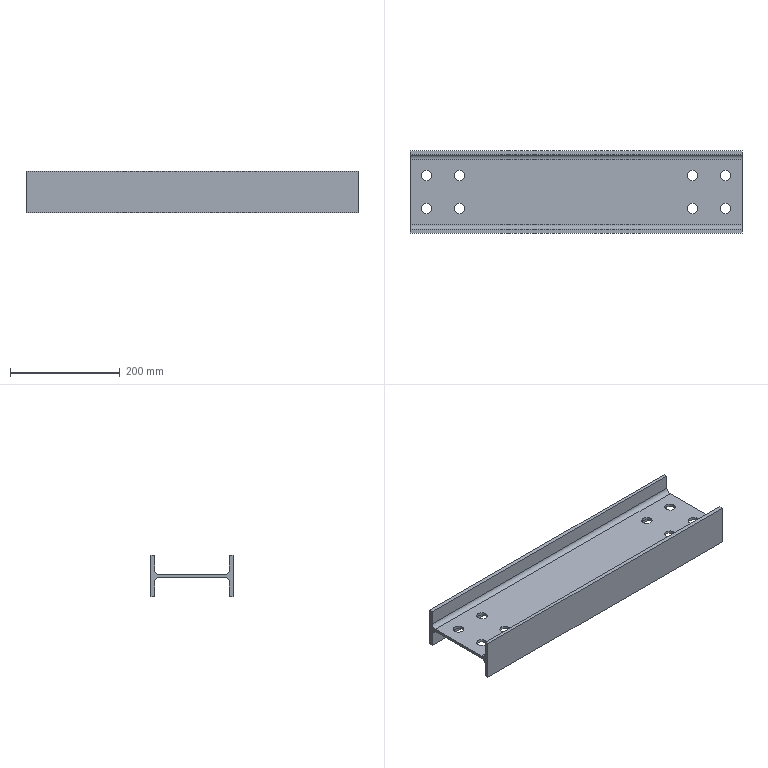Part | STEP file | Metering secondary beam 6_Default<As Machined> | 1 solid | 34 faces | box 605 x 150 x 75 mm | volume 1068546 mm3 | cylinder 20 | plane 14 | commonest cylinder face diameters 19 x16 16 x4